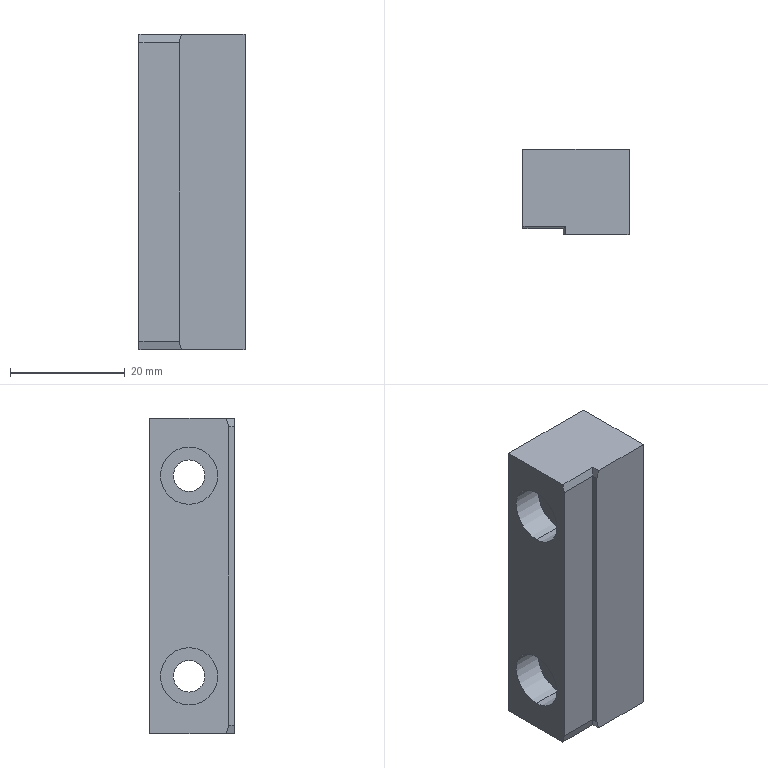Part | STEP file | 11-FG-B03211 | 1 solid | 22 faces | box 18.5 x 14.8 x 55 mm | volume 13198 mm3 | plane 14 | cylinder 8 | commonest cylinder face diameters 5.5 x4 10 x4
STEP:
#1=CARTESIAN_POINT('',(5.4,8.1,40.));
#2=VERTEX_POINT('',#1);
#3=CARTESIAN_POINT('',(5.4,8.1,50.));
#4=VERTEX_POINT('',#3);
#5=CARTESIAN_POINT('',(5.4,8.1,45.));
#6=DIRECTION('',(-1.,0.,0.));
#7=DIRECTION('',(0.,0.,1.));
#8=AXIS2_PLACEMENT_3D('',#5,#6,#7);
#9=CIRCLE('',#8,5.);
#10=EDGE_CURVE('',#2,#4,#9,.T.);
#11=ORIENTED_EDGE('',*,*,#10,.F.);
#12=CARTESIAN_POINT('',(0.,8.1,40.));
#13=VERTEX_POINT('',#12);
#14=CARTESIAN_POINT('',(0.,8.1,40.));
#15=DIRECTION('',(-1.,0.,0.));
#16=VECTOR('',#15,1000.);
#17=LINE('',#14,#16);
#18=EDGE_CURVE('',#2,#13,#17,.T.);
#19=ORIENTED_EDGE('',*,*,#18,.T.);
#20=CARTESIAN_POINT('',(0.,8.1,50.));
#21=VERTEX_POINT('',#20);
#22=CARTESIAN_POINT('',(0.,8.1,45.));
#23=DIRECTION('',(-1.,0.,0.));
#24=DIRECTION('',(0.,0.,1.));
#25=AXIS2_PLACEMENT_3D('',#22,#23,#24);
#26=CIRCLE('',#25,5.);
#27=EDGE_CURVE('',#13,#21,#26,.T.);
#28=ORIENTED_EDGE('',*,*,#27,.T.);
#29=CARTESIAN_POINT('',(0.,8.1,50.));
#30=DIRECTION('',(-1.,0.,0.));
#31=VECTOR('',#30,1000.);
#32=LINE('',#29,#31);
#33=EDGE_CURVE('',#4,#21,#32,.T.);
#34=ORIENTED_EDGE('',*,*,#33,.F.);
#35=EDGE_LOOP('',(#11,#19,#28,#34));
#36=FACE_OUTER_BOUND('',#35,.T.);
#37=CARTESIAN_POINT('',(0.,8.1,45.));
#38=DIRECTION('',(-1.,0.,0.));
#39=DIRECTION('',(0.,0.,1.));
#40=AXIS2_PLACEMENT_3D('',#37,#38,#39);
#41=CYLINDRICAL_SURFACE('',#40,5.);
#42=ADVANCED_FACE('',(#36),#41,.F.);
#43=CARTESIAN_POINT('',(18.5,8.1,42.25));
#44=VERTEX_POINT('',#43);
#45=CARTESIAN_POINT('',(18.5,8.1,47.75));
#46=VERTEX_POINT('',#45);
#47=CARTESIAN_POINT('',(18.5,8.1,45.));
#48=DIRECTION('',(-1.,0.,0.));
#49=DIRECTION('',(0.,0.,1.));
#50=AXIS2_PLACEMENT_3D('',#47,#48,#49);
#51=CIRCLE('',#50,2.75);
#52=EDGE_CURVE('',#44,#46,#51,.T.);
#53=ORIENTED_EDGE('',*,*,#52,.F.);
#54=CARTESIAN_POINT('',(5.4,8.1,42.25));
#55=VERTEX_POINT('',#54);
#56=CARTESIAN_POINT('',(0.,8.1,42.25));
#57=DIRECTION('',(-1.,0.,0.));
#58=VECTOR('',#57,1000.);
#59=LINE('',#56,#58);
#60=EDGE_CURVE('',#44,#55,#59,.T.);
#61=ORIENTED_EDGE('',*,*,#60,.T.);
#62=CARTESIAN_POINT('',(5.4,8.1,47.75));
#63=VERTEX_POINT('',#62);
#64=CARTESIAN_POINT('',(5.4,8.1,45.));
#65=DIRECTION('',(-1.,0.,0.));
#66=DIRECTION('',(0.,0.,1.));
#67=AXIS2_PLACEMENT_3D('',#64,#65,#66);
#68=CIRCLE('',#67,2.75);
#69=EDGE_CURVE('',#55,#63,#68,.T.);
#70=ORIENTED_EDGE('',*,*,#69,.T.);
#71=CARTESIAN_POINT('',(0.,8.1,47.75));
#72=DIRECTION('',(-1.,0.,0.));
#73=VECTOR('',#72,1000.);
#74=LINE('',#71,#73);
#75=EDGE_CURVE('',#46,#63,#74,.T.);
#76=ORIENTED_EDGE('',*,*,#75,.F.);
#77=EDGE_LOOP('',(#53,#61,#70,#76));
#78=FACE_OUTER_BOUND('',#77,.T.);
#79=CARTESIAN_POINT('',(0.,8.1,45.));
#80=DIRECTION('',(-1.,0.,0.));
#81=DIRECTION('',(0.,0.,1.));
#82=AXIS2_PLACEMENT_3D('',#79,#80,#81);
#83=CYLINDRICAL_SURFACE('',#82,2.75);
#84=ADVANCED_FACE('',(#78),#83,.F.);
#85=CARTESIAN_POINT('',(5.4,8.1,5.));
#86=VERTEX_POINT('',#85);
#87=CARTESIAN_POINT('',(5.4,8.1,15.));
#88=VERTEX_POINT('',#87);
#89=CARTESIAN_POINT('',(5.4,8.1,10.));
#90=DIRECTION('',(-1.,0.,0.));
#91=DIRECTION('',(0.,0.,1.));
#92=AXIS2_PLACEMENT_3D('',#89,#90,#91);
#93=CIRCLE('',#92,5.);
#94=EDGE_CURVE('',#86,#88,#93,.T.);
#95=ORIENTED_EDGE('',*,*,#94,.F.);
#96=CARTESIAN_POINT('',(0.,8.1,5.));
#97=VERTEX_POINT('',#96);
#98=CARTESIAN_POINT('',(0.,8.1,5.));
#99=DIRECTION('',(-1.,0.,0.));
#100=VECTOR('',#99,1000.);
#101=LINE('',#98,#100);
#102=EDGE_CURVE('',#86,#97,#101,.T.);
#103=ORIENTED_EDGE('',*,*,#102,.T.);
#104=CARTESIAN_POINT('',(0.,8.1,15.));
#105=VERTEX_POINT('',#104);
#106=CARTESIAN_POINT('',(0.,8.1,10.));
#107=DIRECTION('',(-1.,0.,0.));
#108=DIRECTION('',(0.,0.,1.));
#109=AXIS2_PLACEMENT_3D('',#106,#107,#108);
#110=CIRCLE('',#109,5.);
#111=EDGE_CURVE('',#97,#105,#110,.T.);
#112=ORIENTED_EDGE('',*,*,#111,.T.);
#113=CARTESIAN_POINT('',(0.,8.1,15.));
#114=DIRECTION('',(-1.,0.,0.));
#115=VECTOR('',#114,1000.);
#116=LINE('',#113,#115);
#117=EDGE_CURVE('',#88,#105,#116,.T.);
#118=ORIENTED_EDGE('',*,*,#117,.F.);
#119=EDGE_LOOP('',(#95,#103,#112,#118));
#120=FACE_OUTER_BOUND('',#119,.T.);
#121=CARTESIAN_POINT('',(0.,8.1,10.));
#122=DIRECTION('',(-1.,0.,0.));
#123=DIRECTION('',(0.,0.,1.));
#124=AXIS2_PLACEMENT_3D('',#121,#122,#123);
#125=CYLINDRICAL_SURFACE('',#124,5.);
#126=ADVANCED_FACE('',(#120),#125,.F.);
#127=CARTESIAN_POINT('',(18.5,8.1,7.25));
#128=VERTEX_POINT('',#127);
#129=CARTESIAN_POINT('',(18.5,8.1,12.75));
#130=VERTEX_POINT('',#129);
#131=CARTESIAN_POINT('',(18.5,8.1,10.));
#132=DIRECTION('',(-1.,0.,0.));
#133=DIRECTION('',(0.,0.,1.));
#134=AXIS2_PLACEMENT_3D('',#131,#132,#133);
#135=CIRCLE('',#134,2.75);
#136=EDGE_CURVE('',#128,#130,#135,.T.);
#137=ORIENTED_EDGE('',*,*,#136,.F.);
#138=CARTESIAN_POINT('',(5.4,8.1,7.25));
#139=VERTEX_POINT('',#138);
#140=CARTESIAN_POINT('',(0.,8.1,7.25));
#141=DIRECTION('',(-1.,0.,0.));
#142=VECTOR('',#141,1000.);
#143=LINE('',#140,#142);
#144=EDGE_CURVE('',#128,#139,#143,.T.);
#145=ORIENTED_EDGE('',*,*,#144,.T.);
#146=CARTESIAN_POINT('',(5.4,8.1,12.75));
#147=VERTEX_POINT('',#146);
#148=CARTESIAN_POINT('',(5.4,8.1,10.));
#149=DIRECTION('',(-1.,0.,0.));
#150=DIRECTION('',(0.,0.,1.));
#151=AXIS2_PLACEMENT_3D('',#148,#149,#150);
#152=CIRCLE('',#151,2.75);
#153=EDGE_CURVE('',#139,#147,#152,.T.);
#154=ORIENTED_EDGE('',*,*,#153,.T.);
#155=CARTESIAN_POINT('',(0.,8.1,12.75));
#156=DIRECTION('',(-1.,0.,0.));
#157=VECTOR('',#156,1000.);
#158=LINE('',#155,#157);
#159=EDGE_CURVE('',#130,#147,#158,.T.);
#160=ORIENTED_EDGE('',*,*,#159,.F.);
#161=EDGE_LOOP('',(#137,#145,#154,#160));
#162=FACE_OUTER_BOUND('',#161,.T.);
#163=CARTESIAN_POINT('',(0.,8.1,10.));
#164=DIRECTION('',(-1.,0.,0.));
#165=DIRECTION('',(0.,0.,1.));
#166=AXIS2_PLACEMENT_3D('',#163,#164,#165);
#167=CYLINDRICAL_SURFACE('',#166,2.75);
#168=ADVANCED_FACE('',(#162),#167,.F.);
#169=CARTESIAN_POINT('',(0.,1.2,53.5));
#170=VERTEX_POINT('',#169);
#171=CARTESIAN_POINT('',(0.,1.2,1.5));
#172=VERTEX_POINT('',#171);
#173=CARTESIAN_POINT('',(0.,1.2,55.));
#174=DIRECTION('',(0.,0.,-1.));
#175=VECTOR('',#174,1000.);
#176=LINE('',#173,#175);
#177=EDGE_CURVE('',#170,#172,#176,.T.);
#178=ORIENTED_EDGE('',*,*,#177,.T.);
#179=CARTESIAN_POINT('',(7.,1.2,1.5));
#180=VERTEX_POINT('',#179);
#181=CARTESIAN_POINT('',(7.,1.2,1.5));
#182=DIRECTION('',(1.,0.,0.));
#183=VECTOR('',#182,1000.);
#184=LINE('',#181,#183);
#185=EDGE_CURVE('',#172,#180,#184,.T.);
#186=ORIENTED_EDGE('',*,*,#185,.T.);
#187=CARTESIAN_POINT('',(7.,1.2,53.5));
#188=VERTEX_POINT('',#187);
#189=CARTESIAN_POINT('',(7.,1.2,0.));
#190=DIRECTION('',(0.,0.,-1.));
#191=VECTOR('',#190,1000.);
#192=LINE('',#189,#191);
#193=EDGE_CURVE('',#188,#180,#192,.T.);
#194=ORIENTED_EDGE('',*,*,#193,.F.);
#195=CARTESIAN_POINT('',(0.,1.2,53.5));
#196=DIRECTION('',(-1.,0.,0.));
#197=VECTOR('',#196,1000.);
#198=LINE('',#195,#197);
#199=EDGE_CURVE('',#188,#170,#198,.T.);
#200=ORIENTED_EDGE('',*,*,#199,.T.);
#201=EDGE_LOOP('',(#178,#186,#194,#200));
#202=FACE_OUTER_BOUND('',#201,.T.);
#203=CARTESIAN_POINT('',(0.,1.2,55.));
#204=DIRECTION('',(0.,1.,0.));
#205=DIRECTION('',(-1.,0.,0.));
#206=AXIS2_PLACEMENT_3D('',#203,#204,#205);
#207=PLANE('',#206);
#208=ADVANCED_FACE('',(#202),#207,.F.);
#209=CARTESIAN_POINT('',(0.,8.1,45.));
#210=DIRECTION('',(-1.,0.,0.));
#211=DIRECTION('',(0.,0.,1.));
#212=AXIS2_PLACEMENT_3D('',#209,#210,#211);
#213=CIRCLE('',#212,5.);
#214=EDGE_CURVE('',#21,#13,#213,.T.);
#215=ORIENTED_EDGE('',*,*,#214,.F.);
#216=ORIENTED_EDGE('',*,*,#27,.F.);
#217=EDGE_LOOP('',(#215,#216));
#218=FACE_BOUND('',#217,.T.);
#219=CARTESIAN_POINT('',(0.,8.1,10.));
#220=DIRECTION('',(-1.,0.,0.));
#221=DIRECTION('',(0.,0.,1.));
#222=AXIS2_PLACEMENT_3D('',#219,#220,#221);
#223=CIRCLE('',#222,5.);
#224=EDGE_CURVE('',#105,#97,#223,.T.);
#225=ORIENTED_EDGE('',*,*,#224,.F.);
#226=ORIENTED_EDGE('',*,*,#111,.F.);
#227=EDGE_LOOP('',(#225,#226));
#228=FACE_BOUND('',#227,.T.);
#229=CARTESIAN_POINT('',(0.,15.,0.));
#230=VERTEX_POINT('',#229);
#231=CARTESIAN_POINT('',(0.,1.602,0.));
#232=VERTEX_POINT('',#231);
#233=CARTESIAN_POINT('',(0.,0.,0.));
#234=DIRECTION('',(0.,-1.,0.));
#235=VECTOR('',#234,1000.);
#236=LINE('',#233,#235);
#237=EDGE_CURVE('',#230,#232,#236,.T.);
#238=ORIENTED_EDGE('',*,*,#237,.T.);
#239=CARTESIAN_POINT('',(0.,1.2,1.5));
#240=DIRECTION('',(0.,-0.2588,0.9659));
#241=VECTOR('',#240,1000.);
#242=LINE('',#239,#241);
#243=EDGE_CURVE('',#232,#172,#242,.T.);
#244=ORIENTED_EDGE('',*,*,#243,.T.);
#245=ORIENTED_EDGE('',*,*,#177,.F.);
#246=CARTESIAN_POINT('',(0.,1.602,55.));
#247=VERTEX_POINT('',#246);
#248=CARTESIAN_POINT('',(0.,1.602,55.));
#249=DIRECTION('',(0.,0.2588,0.9659));
#250=VECTOR('',#249,1000.);
#251=LINE('',#248,#250);
#252=EDGE_CURVE('',#170,#247,#251,.T.);
#253=ORIENTED_EDGE('',*,*,#252,.T.);
#254=CARTESIAN_POINT('',(0.,15.,55.));
#255=VERTEX_POINT('',#254);
#256=CARTESIAN_POINT('',(0.,0.,55.));
#257=DIRECTION('',(0.,-1.,0.));
#258=VECTOR('',#257,1000.);
#259=LINE('',#256,#258);
#260=EDGE_CURVE('',#255,#247,#259,.T.);
#261=ORIENTED_EDGE('',*,*,#260,.F.);
#262=CARTESIAN_POINT('',(0.,15.,55.));
#263=DIRECTION('',(0.,0.,-1.));
#264=VECTOR('',#263,1000.);
#265=LINE('',#262,#264);
#266=EDGE_CURVE('',#255,#230,#265,.T.);
#267=ORIENTED_EDGE('',*,*,#266,.T.);
#268=EDGE_LOOP('',(#238,#244,#245,#253,#261,#267));
#269=FACE_OUTER_BOUND('',#268,.T.);
#270=CARTESIAN_POINT('',(0.,0.,55.));
#271=DIRECTION('',(1.,0.,0.));
#272=DIRECTION('',(0.,0.,-1.));
#273=AXIS2_PLACEMENT_3D('',#270,#271,#272);
#274=PLANE('',#273);
#275=ADVANCED_FACE('',(#218,#228,#269),#274,.F.);
#276=CARTESIAN_POINT('',(18.5,8.1,45.));
#277=DIRECTION('',(-1.,0.,0.));
#278=DIRECTION('',(0.,0.,1.));
#279=AXIS2_PLACEMENT_3D('',#276,#277,#278);
#280=CIRCLE('',#279,2.75);
#281=EDGE_CURVE('',#46,#44,#280,.T.);
#282=ORIENTED_EDGE('',*,*,#281,.T.);
#283=ORIENTED_EDGE('',*,*,#52,.T.);
#284=EDGE_LOOP('',(#282,#283));
#285=FACE_BOUND('',#284,.T.);
#286=CARTESIAN_POINT('',(18.5,8.1,10.));
#287=DIRECTION('',(-1.,0.,0.));
#288=DIRECTION('',(0.,0.,1.));
#289=AXIS2_PLACEMENT_3D('',#286,#287,#288);
#290=CIRCLE('',#289,2.75);
#291=EDGE_CURVE('',#130,#128,#290,.T.);
#292=ORIENTED_EDGE('',*,*,#291,.T.);
#293=ORIENTED_EDGE('',*,*,#136,.T.);
#294=EDGE_LOOP('',(#292,#293));
#295=FACE_BOUND('',#294,.T.);
#296=CARTESIAN_POINT('',(18.5,0.2,55.));
#297=VERTEX_POINT('',#296);
#298=CARTESIAN_POINT('',(18.5,15.,55.));
#299=VERTEX_POINT('',#298);
#300=CARTESIAN_POINT('',(18.5,0.,55.));
#301=DIRECTION('',(0.,1.,0.));
#302=VECTOR('',#301,1000.);
#303=LINE('',#300,#302);
#304=EDGE_CURVE('',#297,#299,#303,.T.);
#305=ORIENTED_EDGE('',*,*,#304,.F.);
#306=CARTESIAN_POINT('',(18.5,0.2,0.));
#307=VERTEX_POINT('',#306);
#308=CARTESIAN_POINT('',(18.5,0.2,0.));
#309=DIRECTION('',(0.,0.,1.));
#310=VECTOR('',#309,1000.);
#311=LINE('',#308,#310);
#312=EDGE_CURVE('',#307,#297,#311,.T.);
#313=ORIENTED_EDGE('',*,*,#312,.F.);
#314=CARTESIAN_POINT('',(18.5,15.,0.));
#315=VERTEX_POINT('',#314);
#316=CARTESIAN_POINT('',(18.5,0.,0.));
#317=DIRECTION('',(0.,1.,0.));
#318=VECTOR('',#317,1000.);
#319=LINE('',#316,#318);
#320=EDGE_CURVE('',#307,#315,#319,.T.);
#321=ORIENTED_EDGE('',*,*,#320,.T.);
#322=CARTESIAN_POINT('',(18.5,15.,55.));
#323=DIRECTION('',(0.,0.,-1.));
#324=VECTOR('',#323,1000.);
#325=LINE('',#322,#324);
#326=EDGE_CURVE('',#299,#315,#325,.T.);
#327=ORIENTED_EDGE('',*,*,#326,.F.);
#328=EDGE_LOOP('',(#305,#313,#321,#327));
#329=FACE_OUTER_BOUND('',#328,.T.);
#330=CARTESIAN_POINT('',(18.5,0.,55.));
#331=DIRECTION('',(-1.,0.,0.));
#332=DIRECTION('',(0.,-1.,0.));
#333=AXIS2_PLACEMENT_3D('',#330,#331,#332);
#334=PLANE('',#333);
#335=ADVANCED_FACE('',(#285,#295,#329),#334,.F.);
#336=CARTESIAN_POINT('',(0.,15.,0.));
#337=DIRECTION('',(-1.,0.,0.));
#338=VECTOR('',#337,1000.);
#339=LINE('',#336,#338);
#340=EDGE_CURVE('',#315,#230,#339,.T.);
#341=ORIENTED_EDGE('',*,*,#340,.T.);
#342=ORIENTED_EDGE('',*,*,#266,.F.);
#343=CARTESIAN_POINT('',(0.,15.,55.));
#344=DIRECTION('',(-1.,0.,0.));
#345=VECTOR('',#344,1000.);
#346=LINE('',#343,#345);
#347=EDGE_CURVE('',#299,#255,#346,.T.);
#348=ORIENTED_EDGE('',*,*,#347,.F.);
#349=ORIENTED_EDGE('',*,*,#326,.T.);
#350=EDGE_LOOP('',(#341,#342,#348,#349));
#351=FACE_OUTER_BOUND('',#350,.T.);
#352=CARTESIAN_POINT('',(0.,15.,55.));
#353=DIRECTION('',(0.,-1.,0.));
#354=DIRECTION('',(0.,0.,-1.));
#355=AXIS2_PLACEMENT_3D('',#352,#353,#354);
#356=PLANE('',#355);
#357=ADVANCED_FACE('',(#351),#356,.F.);
#358=CARTESIAN_POINT('',(7.402,1.602,55.));
#359=VERTEX_POINT('',#358);
#360=CARTESIAN_POINT('',(0.,1.602,55.));
#361=DIRECTION('',(1.,0.,0.));
#362=VECTOR('',#361,1000.);
#363=LINE('',#360,#362);
#364=EDGE_CURVE('',#247,#359,#363,.T.);
#365=ORIENTED_EDGE('',*,*,#364,.T.);
#366=CARTESIAN_POINT('',(7.402,0.2,55.));
#367=VERTEX_POINT('',#366);
#368=CARTESIAN_POINT('',(7.402,15.,55.));
#369=DIRECTION('',(0.,-1.,0.));
#370=VECTOR('',#369,1000.);
#371=LINE('',#368,#370);
#372=EDGE_CURVE('',#359,#367,#371,.T.);
#373=ORIENTED_EDGE('',*,*,#372,.T.);
#374=CARTESIAN_POINT('',(18.5,0.2,55.));
#375=DIRECTION('',(-1.,0.,0.));
#376=VECTOR('',#375,1000.);
#377=LINE('',#374,#376);
#378=EDGE_CURVE('',#297,#367,#377,.T.);
#379=ORIENTED_EDGE('',*,*,#378,.F.);
#380=ORIENTED_EDGE('',*,*,#304,.T.);
#381=ORIENTED_EDGE('',*,*,#347,.T.);
#382=ORIENTED_EDGE('',*,*,#260,.T.);
#383=EDGE_LOOP('',(#365,#373,#379,#380,#381,#382));
#384=FACE_OUTER_BOUND('',#383,.T.);
#385=CARTESIAN_POINT('',(0.,15.,55.));
#386=DIRECTION('',(0.,0.,-1.));
#387=DIRECTION('',(-1.,0.,0.));
#388=AXIS2_PLACEMENT_3D('',#385,#386,#387);
#389=PLANE('',#388);
#390=ADVANCED_FACE('',(#384),#389,.F.);
#391=CARTESIAN_POINT('',(7.402,0.2,0.));
#392=VERTEX_POINT('',#391);
#393=CARTESIAN_POINT('',(18.5,0.2,0.));
#394=DIRECTION('',(1.,0.,0.));
#395=VECTOR('',#394,1000.);
#396=LINE('',#393,#395);
#397=EDGE_CURVE('',#392,#307,#396,.T.);
#398=ORIENTED_EDGE('',*,*,#397,.F.);
#399=CARTESIAN_POINT('',(7.402,1.602,0.));
#400=VERTEX_POINT('',#399);
#401=CARTESIAN_POINT('',(7.402,1.2,0.));
#402=DIRECTION('',(0.,1.,0.));
#403=VECTOR('',#402,1000.);
#404=LINE('',#401,#403);
#405=EDGE_CURVE('',#392,#400,#404,.T.);
#406=ORIENTED_EDGE('',*,*,#405,.T.);
#407=CARTESIAN_POINT('',(0.,1.602,0.));
#408=DIRECTION('',(-1.,0.,0.));
#409=VECTOR('',#408,1000.);
#410=LINE('',#407,#409);
#411=EDGE_CURVE('',#400,#232,#410,.T.);
#412=ORIENTED_EDGE('',*,*,#411,.T.);
#413=ORIENTED_EDGE('',*,*,#237,.F.);
#414=ORIENTED_EDGE('',*,*,#340,.F.);
#415=ORIENTED_EDGE('',*,*,#320,.F.);
#416=EDGE_LOOP('',(#398,#406,#412,#413,#414,#415));
#417=FACE_OUTER_BOUND('',#416,.T.);
#418=CARTESIAN_POINT('',(0.,15.,0.));
#419=DIRECTION('',(0.,0.,-1.));
#420=DIRECTION('',(-1.,0.,0.));
#421=AXIS2_PLACEMENT_3D('',#418,#419,#420);
#422=PLANE('',#421);
#423=ADVANCED_FACE('',(#417),#422,.T.);
#424=ORIENTED_EDGE('',*,*,#193,.T.);
#425=CARTESIAN_POINT('',(7.,0.2,1.5));
#426=VERTEX_POINT('',#425);
#427=CARTESIAN_POINT('',(7.,0.2,1.5));
#428=DIRECTION('',(0.,-1.,0.));
#429=VECTOR('',#428,1000.);
#430=LINE('',#427,#429);
#431=EDGE_CURVE('',#180,#426,#430,.T.);
#432=ORIENTED_EDGE('',*,*,#431,.T.);
#433=CARTESIAN_POINT('',(7.,0.2,53.5));
#434=VERTEX_POINT('',#433);
#435=CARTESIAN_POINT('',(7.,0.2,0.));
#436=DIRECTION('',(0.,0.,-1.));
#437=VECTOR('',#436,1000.);
#438=LINE('',#435,#437);
#439=EDGE_CURVE('',#434,#426,#438,.T.);
#440=ORIENTED_EDGE('',*,*,#439,.F.);
#441=CARTESIAN_POINT('',(7.,0.2,53.5));
#442=DIRECTION('',(0.,1.,0.));
#443=VECTOR('',#442,1000.);
#444=LINE('',#441,#443);
#445=EDGE_CURVE('',#434,#188,#444,.T.);
#446=ORIENTED_EDGE('',*,*,#445,.T.);
#447=EDGE_LOOP('',(#424,#432,#440,#446));
#448=FACE_OUTER_BOUND('',#447,.T.);
#449=CARTESIAN_POINT('',(7.,0.2,0.));
#450=DIRECTION('',(1.,0.,0.));
#451=DIRECTION('',(0.,1.,0.));
#452=AXIS2_PLACEMENT_3D('',#449,#450,#451);
#453=PLANE('',#452);
#454=ADVANCED_FACE('',(#448),#453,.F.);
#455=ORIENTED_EDGE('',*,*,#439,.T.);
#456=CARTESIAN_POINT('',(6.906,0.2,1.85));
#457=DIRECTION('',(0.2588,0.,-0.9659));
#458=VECTOR('',#457,1000.);
#459=LINE('',#456,#458);
#460=EDGE_CURVE('',#426,#392,#459,.T.);
#461=ORIENTED_EDGE('',*,*,#460,.T.);
#462=ORIENTED_EDGE('',*,*,#397,.T.);
#463=ORIENTED_EDGE('',*,*,#312,.T.);
#464=ORIENTED_EDGE('',*,*,#378,.T.);
#465=CARTESIAN_POINT('',(-6.844,0.2,1.834));
#466=DIRECTION('',(-0.2588,0.,-0.9659));
#467=VECTOR('',#466,1000.);
#468=LINE('',#465,#467);
#469=EDGE_CURVE('',#367,#434,#468,.T.);
#470=ORIENTED_EDGE('',*,*,#469,.T.);
#471=EDGE_LOOP('',(#455,#461,#462,#463,#464,#470));
#472=FACE_OUTER_BOUND('',#471,.T.);
#473=CARTESIAN_POINT('',(0.,0.2,0.));
#474=DIRECTION('',(0.,-1.,0.));
#475=DIRECTION('',(1.,0.,0.));
#476=AXIS2_PLACEMENT_3D('',#473,#474,#475);
#477=PLANE('',#476);
#478=ADVANCED_FACE('',(#472),#477,.T.);
#479=ORIENTED_EDGE('',*,*,#243,.F.);
#480=ORIENTED_EDGE('',*,*,#411,.F.);
#481=CARTESIAN_POINT('',(8.243,2.443,-3.139));
#482=DIRECTION('',(0.2506,0.2506,-0.9351));
#483=VECTOR('',#482,1000.);
#484=LINE('',#481,#483);
#485=EDGE_CURVE('',#180,#400,#484,.T.);
#486=ORIENTED_EDGE('',*,*,#485,.F.);
#487=ORIENTED_EDGE('',*,*,#185,.F.);
#488=EDGE_LOOP('',(#479,#480,#486,#487));
#489=FACE_OUTER_BOUND('',#488,.T.);
#490=CARTESIAN_POINT('',(0.,1.2,1.5));
#491=DIRECTION('',(0.,-0.9659,-0.2588));
#492=DIRECTION('',(-1.,0.,0.));
#493=AXIS2_PLACEMENT_3D('',#490,#491,#492);
#494=PLANE('',#493);
#495=ADVANCED_FACE('',(#489),#494,.T.);
#496=ORIENTED_EDGE('',*,*,#460,.F.);
#497=ORIENTED_EDGE('',*,*,#431,.F.);
#498=ORIENTED_EDGE('',*,*,#485,.T.);
#499=ORIENTED_EDGE('',*,*,#405,.F.);
#500=EDGE_LOOP('',(#496,#497,#498,#499));
#501=FACE_OUTER_BOUND('',#500,.T.);
#502=CARTESIAN_POINT('',(7.402,15.,0.));
#503=DIRECTION('',(-0.9659,0.,-0.2588));
#504=DIRECTION('',(0.,-1.,0.));
#505=AXIS2_PLACEMENT_3D('',#502,#503,#504);
#506=PLANE('',#505);
#507=ADVANCED_FACE('',(#501),#506,.T.);
#508=ORIENTED_EDGE('',*,*,#252,.F.);
#509=ORIENTED_EDGE('',*,*,#199,.F.);
#510=CARTESIAN_POINT('',(6.937,1.137,53.266));
#511=DIRECTION('',(-0.2506,-0.2506,-0.9351));
#512=VECTOR('',#511,1000.);
#513=LINE('',#510,#512);
#514=EDGE_CURVE('',#359,#188,#513,.T.);
#515=ORIENTED_EDGE('',*,*,#514,.F.);
#516=ORIENTED_EDGE('',*,*,#364,.F.);
#517=EDGE_LOOP('',(#508,#509,#515,#516));
#518=FACE_OUTER_BOUND('',#517,.T.);
#519=CARTESIAN_POINT('',(0.,1.602,55.));
#520=DIRECTION('',(0.,0.9659,-0.2588));
#521=DIRECTION('',(1.,0.,0.));
#522=AXIS2_PLACEMENT_3D('',#519,#520,#521);
#523=PLANE('',#522);
#524=ADVANCED_FACE('',(#518),#523,.F.);
#525=ORIENTED_EDGE('',*,*,#469,.F.);
#526=ORIENTED_EDGE('',*,*,#372,.F.);
#527=ORIENTED_EDGE('',*,*,#514,.T.);
#528=ORIENTED_EDGE('',*,*,#445,.F.);
#529=EDGE_LOOP('',(#525,#526,#527,#528));
#530=FACE_OUTER_BOUND('',#529,.T.);
#531=CARTESIAN_POINT('',(7.,0.2,53.5));
#532=DIRECTION('',(0.9659,0.,-0.2588));
#533=DIRECTION('',(0.,1.,0.));
#534=AXIS2_PLACEMENT_3D('',#531,#532,#533);
#535=PLANE('',#534);
#536=ADVANCED_FACE('',(#530),#535,.F.);
#537=ORIENTED_EDGE('',*,*,#144,.F.);
#538=ORIENTED_EDGE('',*,*,#291,.F.);
#539=ORIENTED_EDGE('',*,*,#159,.T.);
#540=CARTESIAN_POINT('',(5.4,8.1,10.));
#541=DIRECTION('',(-1.,0.,0.));
#542=DIRECTION('',(0.,0.,1.));
#543=AXIS2_PLACEMENT_3D('',#540,#541,#542);
#544=CIRCLE('',#543,2.75);
#545=EDGE_CURVE('',#147,#139,#544,.T.);
#546=ORIENTED_EDGE('',*,*,#545,.T.);
#547=EDGE_LOOP('',(#537,#538,#539,#546));
#548=FACE_OUTER_BOUND('',#547,.T.);
#549=CARTESIAN_POINT('',(0.,8.1,10.));
#550=DIRECTION('',(-1.,0.,0.));
#551=DIRECTION('',(0.,0.,1.));
#552=AXIS2_PLACEMENT_3D('',#549,#550,#551);
#553=CYLINDRICAL_SURFACE('',#552,2.75);
#554=ADVANCED_FACE('',(#548),#553,.F.);
#555=ORIENTED_EDGE('',*,*,#545,.F.);
#556=ORIENTED_EDGE('',*,*,#153,.F.);
#557=EDGE_LOOP('',(#555,#556));
#558=FACE_BOUND('',#557,.T.);
#559=CARTESIAN_POINT('',(5.4,8.1,10.));
#560=DIRECTION('',(-1.,0.,0.));
#561=DIRECTION('',(0.,0.,1.));
#562=AXIS2_PLACEMENT_3D('',#559,#560,#561);
#563=CIRCLE('',#562,5.);
#564=EDGE_CURVE('',#88,#86,#563,.T.);
#565=ORIENTED_EDGE('',*,*,#564,.T.);
#566=ORIENTED_EDGE('',*,*,#94,.T.);
#567=EDGE_LOOP('',(#565,#566));
#568=FACE_OUTER_BOUND('',#567,.T.);
#569=CARTESIAN_POINT('',(5.4,10.85,10.));
#570=DIRECTION('',(1.,0.,0.));
#571=DIRECTION('',(0.,0.,-1.));
#572=AXIS2_PLACEMENT_3D('',#569,#570,#571);
#573=PLANE('',#572);
#574=ADVANCED_FACE('',(#558,#568),#573,.F.);
#575=ORIENTED_EDGE('',*,*,#102,.F.);
#576=ORIENTED_EDGE('',*,*,#564,.F.);
#577=ORIENTED_EDGE('',*,*,#117,.T.);
#578=ORIENTED_EDGE('',*,*,#224,.T.);
#579=EDGE_LOOP('',(#575,#576,#577,#578));
#580=FACE_OUTER_BOUND('',#579,.T.);
#581=CARTESIAN_POINT('',(0.,8.1,10.));
#582=DIRECTION('',(-1.,0.,0.));
#583=DIRECTION('',(0.,0.,1.));
#584=AXIS2_PLACEMENT_3D('',#581,#582,#583);
#585=CYLINDRICAL_SURFACE('',#584,5.);
#586=ADVANCED_FACE('',(#580),#585,.F.);
#587=ORIENTED_EDGE('',*,*,#60,.F.);
#588=ORIENTED_EDGE('',*,*,#281,.F.);
#589=ORIENTED_EDGE('',*,*,#75,.T.);
#590=CARTESIAN_POINT('',(5.4,8.1,45.));
#591=DIRECTION('',(-1.,0.,0.));
#592=DIRECTION('',(0.,0.,1.));
#593=AXIS2_PLACEMENT_3D('',#590,#591,#592);
#594=CIRCLE('',#593,2.75);
#595=EDGE_CURVE('',#63,#55,#594,.T.);
#596=ORIENTED_EDGE('',*,*,#595,.T.);
#597=EDGE_LOOP('',(#587,#588,#589,#596));
#598=FACE_OUTER_BOUND('',#597,.T.);
#599=CARTESIAN_POINT('',(0.,8.1,45.));
#600=DIRECTION('',(-1.,0.,0.));
#601=DIRECTION('',(0.,0.,1.));
#602=AXIS2_PLACEMENT_3D('',#599,#600,#601);
#603=CYLINDRICAL_SURFACE('',#602,2.75);
#604=ADVANCED_FACE('',(#598),#603,.F.);
#605=ORIENTED_EDGE('',*,*,#595,.F.);
#606=ORIENTED_EDGE('',*,*,#69,.F.);
#607=EDGE_LOOP('',(#605,#606));
#608=FACE_BOUND('',#607,.T.);
#609=CARTESIAN_POINT('',(5.4,8.1,45.));
#610=DIRECTION('',(-1.,0.,0.));
#611=DIRECTION('',(0.,0.,1.));
#612=AXIS2_PLACEMENT_3D('',#609,#610,#611);
#613=CIRCLE('',#612,5.);
#614=EDGE_CURVE('',#4,#2,#613,.T.);
#615=ORIENTED_EDGE('',*,*,#614,.T.);
#616=ORIENTED_EDGE('',*,*,#10,.T.);
#617=EDGE_LOOP('',(#615,#616));
#618=FACE_OUTER_BOUND('',#617,.T.);
#619=CARTESIAN_POINT('',(5.4,10.85,45.));
#620=DIRECTION('',(1.,0.,0.));
#621=DIRECTION('',(0.,0.,-1.));
#622=AXIS2_PLACEMENT_3D('',#619,#620,#621);
#623=PLANE('',#622);
#624=ADVANCED_FACE('',(#608,#618),#623,.F.);
#625=ORIENTED_EDGE('',*,*,#18,.F.);
#626=ORIENTED_EDGE('',*,*,#614,.F.);
#627=ORIENTED_EDGE('',*,*,#33,.T.);
#628=ORIENTED_EDGE('',*,*,#214,.T.);
#629=EDGE_LOOP('',(#625,#626,#627,#628));
#630=FACE_OUTER_BOUND('',#629,.T.);
#631=CARTESIAN_POINT('',(0.,8.1,45.));
#632=DIRECTION('',(-1.,0.,0.));
#633=DIRECTION('',(0.,0.,1.));
#634=AXIS2_PLACEMENT_3D('',#631,#632,#633);
#635=CYLINDRICAL_SURFACE('',#634,5.);
#636=ADVANCED_FACE('',(#630),#635,.F.);
#637=CLOSED_SHELL('',(#42,#84,#126,#168,#208,#275,#335,#357,#390,#423,#454,#478,#495,#507,#524,#536,#554,#574,#586,#604,#624,#636));
#638=MANIFOLD_SOLID_BREP('',#637);
#639=CARTESIAN_POINT('',(0.,0.,0.));
#640=DIRECTION('',(0.,0.,1.));
#641=DIRECTION('',(1.,0.,0.));
#642=AXIS2_PLACEMENT_3D('',#639,#640,#641);
#643=(LENGTH_UNIT()NAMED_UNIT(*)SI_UNIT(.MILLI.,.METRE.));
#644=UNCERTAINTY_MEASURE_WITH_UNIT(LENGTH_MEASURE(0.00001),#643,'','');
#645=(NAMED_UNIT(*)PLANE_ANGLE_UNIT()SI_UNIT($,.RADIAN.));
#646=(NAMED_UNIT(*)SI_UNIT($,.STERADIAN.)SOLID_ANGLE_UNIT());
#647=(GEOMETRIC_REPRESENTATION_CONTEXT(3)GLOBAL_UNCERTAINTY_ASSIGNED_CONTEXT((#644))GLOBAL_UNIT_ASSIGNED_CONTEXT((#643,#645,#646))REPRESENTATION_CONTEXT('',''));
#648=ADVANCED_BREP_SHAPE_REPRESENTATION('',(#638,#642),#647);